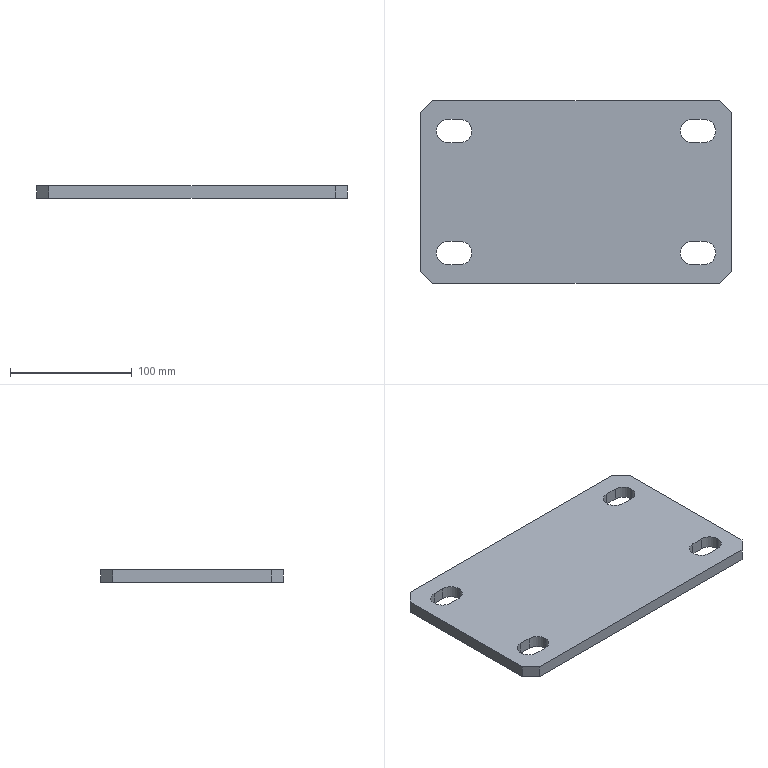Part | STEP file | E3-Bracket连接Plate 1 | 1 solid | 30 faces | box 255 x 150 x 10 mm | volume 361559 mm3 | plane 18 | cylinder 12 | commonest cylinder face diameters 19 x12